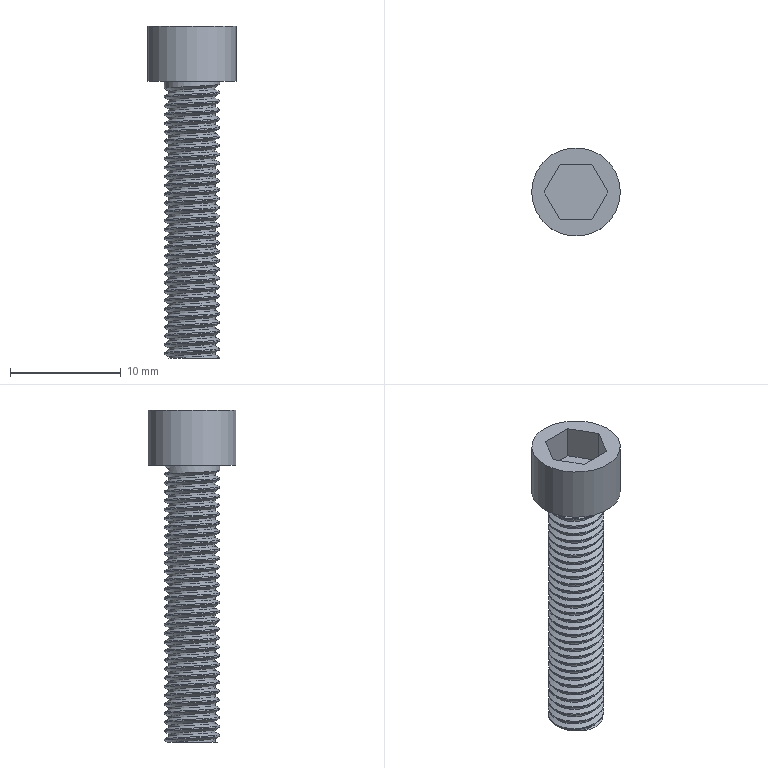Part | NX | features DATUM_CSYS 4, EXTRUDE 3, SKETCH 3, THREADS 1 | 1 solid | 17 faces | box 8 x 8 x 30 mm | volume 577.822 mm3 | plane 11 | cylinder 3 | spline 3 | commonest cylinder face diameters 4.2 x1 5 x1 8 x1